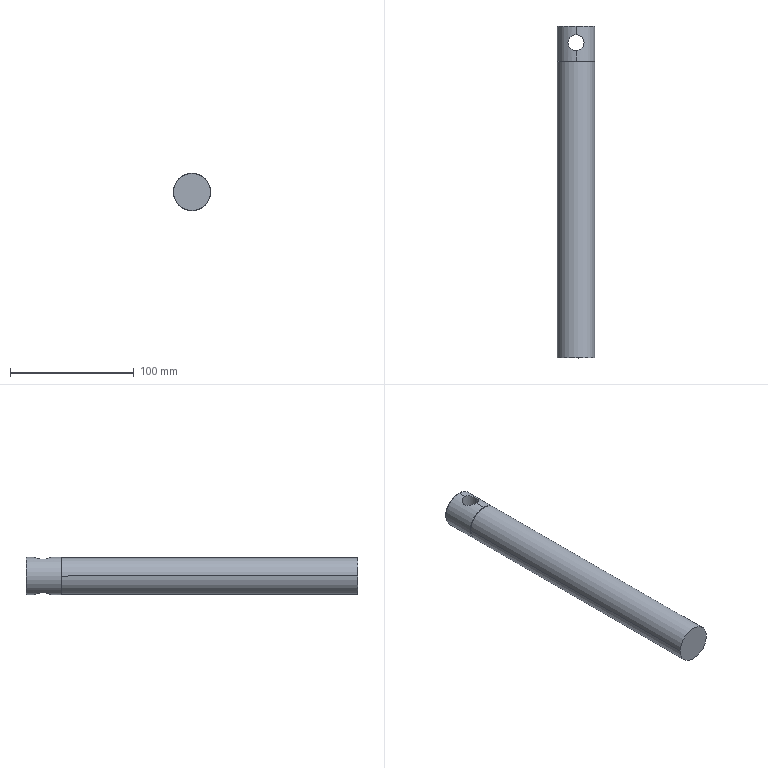Part | SolidWorks | features BaseBody 1 | 1 solid | 29 faces | box 30 x 268.629 x 30.034 mm | volume 178824 mm3 | cylinder 14 | plane 7 | cone 6 | torus 2 | commonest cylinder face diameters 26 x4 30 x4 13 x2 18 x2 24 x2
STEP:
#1=CARTESIAN_POINT('',(406.073,347.307,68.537));
#2=VERTEX_POINT('',#1);
#3=CARTESIAN_POINT('',(391.077,347.309,83.541));
#4=VERTEX_POINT('',#3);
#5=CARTESIAN_POINT('',(406.077,347.309,83.537));
#6=DIRECTION('',(-0.000000041,1.,-0.0001428));
#7=DIRECTION('',(-1.,0.,0.0002857));
#8=AXIS2_PLACEMENT_3D('',#5,#6,#7);
#9=CIRCLE('',#8,15.);
#10=EDGE_CURVE('',#2,#4,#9,.T.);
#11=ORIENTED_EDGE('',*,*,#10,.T.);
#12=CARTESIAN_POINT('',(391.577,347.809,83.541));
#13=VERTEX_POINT('',#12);
#14=CARTESIAN_POINT('',(391.577,347.309,83.541));
#15=DIRECTION('',(-0.0002857,-0.0001428,-1.));
#16=DIRECTION('',(-1.,0.,0.0002857));
#17=AXIS2_PLACEMENT_3D('',#14,#15,#16);
#18=CIRCLE('',#17,0.5);
#19=EDGE_CURVE('',#4,#13,#18,.T.);
#20=ORIENTED_EDGE('',*,*,#19,.T.);
#21=CARTESIAN_POINT('',(420.577,347.809,83.533));
#22=VERTEX_POINT('',#21);
#23=CARTESIAN_POINT('',(406.077,347.809,83.537));
#24=DIRECTION('',(-0.000000041,1.,-0.0001428));
#25=DIRECTION('',(1.,0.,-0.0002857));
#26=AXIS2_PLACEMENT_3D('',#23,#24,#25);
#27=CIRCLE('',#26,14.5);
#28=EDGE_CURVE('',#22,#13,#27,.T.);
#29=ORIENTED_EDGE('',*,*,#28,.F.);
#30=CARTESIAN_POINT('',(421.077,347.309,83.533));
#31=VERTEX_POINT('',#30);
#32=CARTESIAN_POINT('',(420.577,347.309,83.533));
#33=DIRECTION('',(0.0002857,0.0001428,1.));
#34=DIRECTION('',(1.,0.,-0.0002857));
#35=AXIS2_PLACEMENT_3D('',#32,#33,#34);
#36=CIRCLE('',#35,0.5);
#37=EDGE_CURVE('',#31,#22,#36,.T.);
#38=ORIENTED_EDGE('',*,*,#37,.F.);
#39=CARTESIAN_POINT('',(406.077,347.309,83.537));
#40=DIRECTION('',(-0.000000041,1.,-0.0001428));
#41=DIRECTION('',(-1.,0.,0.0002857));
#42=AXIS2_PLACEMENT_3D('',#39,#40,#41);
#43=CIRCLE('',#42,15.);
#44=EDGE_CURVE('',#31,#2,#43,.T.);
#45=ORIENTED_EDGE('',*,*,#44,.T.);
#46=EDGE_LOOP('',(#11,#20,#29,#38,#45));
#47=FACE_OUTER_BOUND('',#46,.T.);
#48=CARTESIAN_POINT('',(406.077,347.309,83.537));
#49=DIRECTION('',(-0.000000041,1.,-0.0001428));
#50=DIRECTION('',(1.,0.,-0.0002857));
#51=AXIS2_PLACEMENT_3D('',#48,#49,#50);
#52=TOROIDAL_SURFACE('',#51,14.5,0.5);
#53=ADVANCED_FACE('',(#47),#52,.T.);
#54=CARTESIAN_POINT('',(406.073,340.807,68.538));
#55=VERTEX_POINT('',#54);
#56=CARTESIAN_POINT('',(412.574,334.308,70.018));
#57=VERTEX_POINT('',#56);
#58=CARTESIAN_POINT('',(406.073,340.807,68.538));
#59=CARTESIAN_POINT('',(406.508,340.807,68.538));
#60=CARTESIAN_POINT('',(406.937,340.764,68.556));
#61=CARTESIAN_POINT('',(407.571,340.636,68.611));
#62=CARTESIAN_POINT('',(407.781,340.583,68.633));
#63=CARTESIAN_POINT('',(408.191,340.457,68.686));
#64=CARTESIAN_POINT('',(408.39,340.384,68.716));
#65=CARTESIAN_POINT('',(408.976,340.139,68.815));
#66=CARTESIAN_POINT('',(409.349,339.938,68.895));
#67=CARTESIAN_POINT('',(410.054,339.463,69.07));
#68=CARTESIAN_POINT('',(410.378,339.196,69.164));
#69=CARTESIAN_POINT('',(410.821,338.752,69.307));
#70=CARTESIAN_POINT('',(410.962,338.596,69.355));
#71=CARTESIAN_POINT('',(411.23,338.27,69.45));
#72=CARTESIAN_POINT('',(411.357,338.1,69.497));
#73=CARTESIAN_POINT('',(411.708,337.575,69.633));
#74=CARTESIAN_POINT('',(411.907,337.205,69.716));
#75=CARTESIAN_POINT('',(412.234,336.423,69.859));
#76=CARTESIAN_POINT('',(412.362,336.008,69.918));
#77=CARTESIAN_POINT('',(412.53,335.17,69.997));
#78=CARTESIAN_POINT('',(412.574,334.743,70.018));
#79=CARTESIAN_POINT('',(412.574,334.308,70.018));
#80=B_SPLINE_CURVE_WITH_KNOTS('',3,(#58,#59,#60,#61,#62,#63,#64,#65,#66,#67,#68,#69,#70,#71,#72,#73,#74,#75,#76,#77,#78,#79),.UNSPECIFIED.,.F.,.F.,(4,2,2,2,2,2,2,2,2,2,4),(0.01028,0.01157,0.01221,0.01285,0.01414,0.01543,0.01607,0.01671,0.018,0.01928,0.02057),.UNSPECIFIED.);
#81=EDGE_CURVE('',#55,#57,#80,.T.);
#82=ORIENTED_EDGE('',*,*,#81,.T.);
#83=CARTESIAN_POINT('',(412.581,334.311,97.055));
#84=VERTEX_POINT('',#83);
#85=CARTESIAN_POINT('',(412.573,334.307,69.287));
#86=DIRECTION('',(0.0002857,0.0001428,1.));
#87=VECTOR('',#86,1000.);
#88=LINE('',#85,#87);
#89=EDGE_CURVE('',#57,#84,#88,.T.);
#90=ORIENTED_EDGE('',*,*,#89,.T.);
#91=CARTESIAN_POINT('',(406.082,340.812,98.538));
#92=VERTEX_POINT('',#91);
#93=CARTESIAN_POINT('',(412.581,334.311,97.055));
#94=CARTESIAN_POINT('',(412.581,334.747,97.055));
#95=CARTESIAN_POINT('',(412.538,335.173,97.076));
#96=CARTESIAN_POINT('',(412.37,336.011,97.155));
#97=CARTESIAN_POINT('',(412.243,336.426,97.214));
#98=CARTESIAN_POINT('',(411.915,337.209,97.357));
#99=CARTESIAN_POINT('',(411.716,337.58,97.441));
#100=CARTESIAN_POINT('',(411.363,338.107,97.577));
#101=CARTESIAN_POINT('',(411.236,338.277,97.624));
#102=CARTESIAN_POINT('',(410.968,338.602,97.719));
#103=CARTESIAN_POINT('',(410.828,338.758,97.767));
#104=CARTESIAN_POINT('',(410.384,339.201,97.91));
#105=CARTESIAN_POINT('',(410.059,339.47,98.004));
#106=CARTESIAN_POINT('',(409.355,339.943,98.18));
#107=CARTESIAN_POINT('',(408.984,340.143,98.259));
#108=CARTESIAN_POINT('',(408.398,340.388,98.358));
#109=CARTESIAN_POINT('',(408.199,340.461,98.389));
#110=CARTESIAN_POINT('',(407.789,340.587,98.441));
#111=CARTESIAN_POINT('',(407.578,340.641,98.464));
#112=CARTESIAN_POINT('',(406.945,340.768,98.519));
#113=CARTESIAN_POINT('',(406.517,340.812,98.538));
#114=CARTESIAN_POINT('',(406.082,340.812,98.538));
#115=B_SPLINE_CURVE_WITH_KNOTS('',3,(#93,#94,#95,#96,#97,#98,#99,#100,#101,#102,#103,#104,#105,#106,#107,#108,#109,#110,#111,#112,#113,#114),.UNSPECIFIED.,.F.,.F.,(4,2,2,2,2,2,2,2,2,2,4),(-0.02056,-0.01928,-0.01799,-0.01671,-0.01606,-0.01542,-0.01414,-0.01285,-0.01221,-0.01156,-0.01028),.UNSPECIFIED.);
#116=EDGE_CURVE('',#84,#92,#115,.T.);
#117=ORIENTED_EDGE('',*,*,#116,.T.);
#118=CARTESIAN_POINT('',(399.581,334.311,97.059));
#119=VERTEX_POINT('',#118);
#120=CARTESIAN_POINT('',(406.082,340.812,98.538));
#121=CARTESIAN_POINT('',(405.647,340.812,98.538));
#122=CARTESIAN_POINT('',(405.221,340.768,98.519));
#123=CARTESIAN_POINT('',(404.592,340.642,98.466));
#124=CARTESIAN_POINT('',(404.385,340.59,98.443));
#125=CARTESIAN_POINT('',(403.974,340.464,98.391));
#126=CARTESIAN_POINT('',(403.772,340.391,98.361));
#127=CARTESIAN_POINT('',(403.183,340.145,98.261));
#128=CARTESIAN_POINT('',(402.812,339.945,98.183));
#129=CARTESIAN_POINT('',(402.11,339.474,98.008));
#130=CARTESIAN_POINT('',(401.779,339.202,97.912));
#131=CARTESIAN_POINT('',(401.184,338.606,97.721));
#132=CARTESIAN_POINT('',(400.919,338.283,97.625));
#133=CARTESIAN_POINT('',(400.451,337.586,97.445));
#134=CARTESIAN_POINT('',(400.247,337.208,97.36));
#135=CARTESIAN_POINT('',(399.921,336.427,97.218));
#136=CARTESIAN_POINT('',(399.796,336.022,97.16));
#137=CARTESIAN_POINT('',(399.668,335.392,97.1));
#138=CARTESIAN_POINT('',(399.636,335.176,97.085));
#139=CARTESIAN_POINT('',(399.592,334.745,97.064));
#140=CARTESIAN_POINT('',(399.581,334.529,97.059));
#141=CARTESIAN_POINT('',(399.581,334.311,97.059));
#142=B_SPLINE_CURVE_WITH_KNOTS('',3,(#120,#121,#122,#123,#124,#125,#126,#127,#128,#129,#130,#131,#132,#133,#134,#135,#136,#137,#138,#139,#140,#141),.UNSPECIFIED.,.F.,.F.,(4,2,2,2,2,2,2,2,2,2,4),(-0.01028,-0.008994,-0.008351,-0.007709,-0.006424,-0.005139,-0.003854,-0.00257,-0.001285,-0.0006424,0.),.UNSPECIFIED.);
#143=EDGE_CURVE('',#92,#119,#142,.T.);
#144=ORIENTED_EDGE('',*,*,#143,.T.);
#145=CARTESIAN_POINT('',(399.574,334.308,70.022));
#146=VERTEX_POINT('',#145);
#147=CARTESIAN_POINT('',(399.573,334.307,69.291));
#148=DIRECTION('',(0.0002857,0.0001428,1.));
#149=VECTOR('',#148,1000.);
#150=LINE('',#147,#149);
#151=EDGE_CURVE('',#146,#119,#150,.T.);
#152=ORIENTED_EDGE('',*,*,#151,.F.);
#153=CARTESIAN_POINT('',(399.574,334.308,70.022));
#154=CARTESIAN_POINT('',(399.574,334.743,70.022));
#155=CARTESIAN_POINT('',(399.617,335.169,70.001));
#156=CARTESIAN_POINT('',(399.785,336.007,69.922));
#157=CARTESIAN_POINT('',(399.912,336.422,69.863));
#158=CARTESIAN_POINT('',(400.24,337.205,69.72));
#159=CARTESIAN_POINT('',(400.439,337.576,69.636));
#160=CARTESIAN_POINT('',(400.792,338.103,69.5));
#161=CARTESIAN_POINT('',(400.919,338.273,69.452));
#162=CARTESIAN_POINT('',(401.186,338.598,69.357));
#163=CARTESIAN_POINT('',(401.327,338.753,69.309));
#164=CARTESIAN_POINT('',(401.771,339.197,69.166));
#165=CARTESIAN_POINT('',(402.096,339.466,69.071));
#166=CARTESIAN_POINT('',(402.8,339.939,68.896));
#167=CARTESIAN_POINT('',(403.171,340.139,68.817));
#168=CARTESIAN_POINT('',(403.757,340.384,68.717));
#169=CARTESIAN_POINT('',(403.956,340.457,68.687));
#170=CARTESIAN_POINT('',(404.366,340.583,68.634));
#171=CARTESIAN_POINT('',(404.577,340.636,68.612));
#172=CARTESIAN_POINT('',(405.21,340.764,68.557));
#173=CARTESIAN_POINT('',(405.638,340.807,68.538));
#174=CARTESIAN_POINT('',(406.073,340.807,68.538));
#175=B_SPLINE_CURVE_WITH_KNOTS('',3,(#153,#154,#155,#156,#157,#158,#159,#160,#161,#162,#163,#164,#165,#166,#167,#168,#169,#170,#171,#172,#173,#174),.UNSPECIFIED.,.F.,.F.,(4,2,2,2,2,2,2,2,2,2,4),(-0.000000012,0.001285,0.002571,0.003856,0.004499,0.005142,0.006427,0.007713,0.008355,0.008998,0.01028),.UNSPECIFIED.);
#176=EDGE_CURVE('',#146,#55,#175,.T.);
#177=ORIENTED_EDGE('',*,*,#176,.T.);
#178=EDGE_LOOP('',(#82,#90,#117,#144,#152,#177));
#179=FACE_OUTER_BOUND('',#178,.T.);
#180=CARTESIAN_POINT('',(406.073,334.307,69.289));
#181=DIRECTION('',(0.0002857,0.0001428,1.));
#182=DIRECTION('',(-1.,0.,0.0002857));
#183=AXIS2_PLACEMENT_3D('',#180,#181,#182);
#184=CYLINDRICAL_SURFACE('',#183,6.5);
#185=ADVANCED_FACE('',(#179),#184,.F.);
#186=ORIENTED_EDGE('',*,*,#10,.F.);
#187=CARTESIAN_POINT('',(406.073,336.807,68.538));
#188=DIRECTION('',(0.000000041,-1.,0.0001428));
#189=VECTOR('',#188,1000.);
#190=LINE('',#187,#189);
#191=EDGE_CURVE('',#2,#55,#190,.T.);
#192=ORIENTED_EDGE('',*,*,#191,.T.);
#193=ORIENTED_EDGE('',*,*,#176,.F.);
#194=CARTESIAN_POINT('',(406.073,327.807,68.54));
#195=VERTEX_POINT('',#194);
#196=CARTESIAN_POINT('',(406.073,327.807,68.54));
#197=CARTESIAN_POINT('',(405.638,327.807,68.54));
#198=CARTESIAN_POINT('',(405.209,327.851,68.559));
#199=CARTESIAN_POINT('',(404.575,327.979,68.613));
#200=CARTESIAN_POINT('',(404.365,328.032,68.636));
#201=CARTESIAN_POINT('',(403.956,328.158,68.689));
#202=CARTESIAN_POINT('',(403.756,328.231,68.719));
#203=CARTESIAN_POINT('',(403.17,328.476,68.819));
#204=CARTESIAN_POINT('',(402.797,328.677,68.898));
#205=CARTESIAN_POINT('',(402.092,329.152,69.074));
#206=CARTESIAN_POINT('',(401.769,329.419,69.168));
#207=CARTESIAN_POINT('',(401.326,329.863,69.311));
#208=CARTESIAN_POINT('',(401.185,330.019,69.359));
#209=CARTESIAN_POINT('',(400.917,330.345,69.454));
#210=CARTESIAN_POINT('',(400.79,330.516,69.501));
#211=CARTESIAN_POINT('',(400.439,331.04,69.637));
#212=CARTESIAN_POINT('',(400.24,331.41,69.72));
#213=CARTESIAN_POINT('',(399.913,332.192,69.863));
#214=CARTESIAN_POINT('',(399.785,332.608,69.922));
#215=CARTESIAN_POINT('',(399.617,333.446,70.001));
#216=CARTESIAN_POINT('',(399.574,333.872,70.022));
#217=CARTESIAN_POINT('',(399.574,334.308,70.022));
#218=B_SPLINE_CURVE_WITH_KNOTS('',3,(#196,#197,#198,#199,#200,#201,#202,#203,#204,#205,#206,#207,#208,#209,#210,#211,#212,#213,#214,#215,#216,#217),.UNSPECIFIED.,.F.,.F.,(4,2,2,2,2,2,2,2,2,2,4),(-0.01029,-0.009,-0.008357,-0.007714,-0.006429,-0.005143,-0.0045,-0.003857,-0.002571,-0.001286,-0.000000012),.UNSPECIFIED.);
#219=EDGE_CURVE('',#195,#146,#218,.T.);
#220=ORIENTED_EDGE('',*,*,#219,.F.);
#221=CARTESIAN_POINT('',(406.073,319.307,68.541));
#222=VERTEX_POINT('',#221);
#223=CARTESIAN_POINT('',(406.073,336.807,68.538));
#224=DIRECTION('',(0.000000041,-1.,0.0001428));
#225=VECTOR('',#224,1000.);
#226=LINE('',#223,#225);
#227=EDGE_CURVE('',#195,#222,#226,.T.);
#228=ORIENTED_EDGE('',*,*,#227,.T.);
#229=CARTESIAN_POINT('',(391.077,319.309,83.545));
#230=VERTEX_POINT('',#229);
#231=CARTESIAN_POINT('',(406.077,319.309,83.541));
#232=DIRECTION('',(0.000000041,-1.,0.0001428));
#233=DIRECTION('',(-0.0002857,-0.0001428,-1.));
#234=AXIS2_PLACEMENT_3D('',#231,#232,#233);
#235=CIRCLE('',#234,15.);
#236=EDGE_CURVE('',#230,#222,#235,.T.);
#237=ORIENTED_EDGE('',*,*,#236,.F.);
#238=CARTESIAN_POINT('',(406.082,319.312,98.541));
#239=VERTEX_POINT('',#238);
#240=CARTESIAN_POINT('',(406.077,319.309,83.541));
#241=DIRECTION('',(0.000000041,-1.,0.0001428));
#242=DIRECTION('',(-0.0002857,-0.0001428,-1.));
#243=AXIS2_PLACEMENT_3D('',#240,#241,#242);
#244=CIRCLE('',#243,15.);
#245=EDGE_CURVE('',#239,#230,#244,.T.);
#246=ORIENTED_EDGE('',*,*,#245,.F.);
#247=CARTESIAN_POINT('',(406.082,327.812,98.54));
#248=VERTEX_POINT('',#247);
#249=CARTESIAN_POINT('',(406.082,336.812,98.538));
#250=DIRECTION('',(0.000000041,-1.,0.0001428));
#251=VECTOR('',#250,1000.);
#252=LINE('',#249,#251);
#253=EDGE_CURVE('',#248,#239,#252,.T.);
#254=ORIENTED_EDGE('',*,*,#253,.F.);
#255=CARTESIAN_POINT('',(399.581,334.311,97.059));
#256=CARTESIAN_POINT('',(399.581,333.876,97.059));
#257=CARTESIAN_POINT('',(399.625,333.45,97.08));
#258=CARTESIAN_POINT('',(399.793,332.612,97.159));
#259=CARTESIAN_POINT('',(399.92,332.197,97.218));
#260=CARTESIAN_POINT('',(400.248,331.414,97.361));
#261=CARTESIAN_POINT('',(400.447,331.043,97.445));
#262=CARTESIAN_POINT('',(400.8,330.516,97.581));
#263=CARTESIAN_POINT('',(400.927,330.346,97.628));
#264=CARTESIAN_POINT('',(401.195,330.021,97.723));
#265=CARTESIAN_POINT('',(401.335,329.866,97.771));
#266=CARTESIAN_POINT('',(401.779,329.422,97.914));
#267=CARTESIAN_POINT('',(402.104,329.153,98.008));
#268=CARTESIAN_POINT('',(402.809,328.68,98.183));
#269=CARTESIAN_POINT('',(403.18,328.48,98.262));
#270=CARTESIAN_POINT('',(403.765,328.235,98.362));
#271=CARTESIAN_POINT('',(403.965,328.162,98.391));
#272=CARTESIAN_POINT('',(404.375,328.036,98.444));
#273=CARTESIAN_POINT('',(404.585,327.983,98.467));
#274=CARTESIAN_POINT('',(405.218,327.855,98.521));
#275=CARTESIAN_POINT('',(405.647,327.812,98.54));
#276=CARTESIAN_POINT('',(406.082,327.812,98.54));
#277=B_SPLINE_CURVE_WITH_KNOTS('',3,(#255,#256,#257,#258,#259,#260,#261,#262,#263,#264,#265,#266,#267,#268,#269,#270,#271,#272,#273,#274,#275,#276),.UNSPECIFIED.,.F.,.F.,(4,2,2,2,2,2,2,2,2,2,4),(0.,0.001285,0.002571,0.003856,0.004499,0.005142,0.006427,0.007713,0.008355,0.008998,0.01028),.UNSPECIFIED.);
#278=EDGE_CURVE('',#119,#248,#277,.T.);
#279=ORIENTED_EDGE('',*,*,#278,.F.);
#280=ORIENTED_EDGE('',*,*,#143,.F.);
#281=CARTESIAN_POINT('',(406.082,347.312,98.537));
#282=VERTEX_POINT('',#281);
#283=CARTESIAN_POINT('',(406.082,336.812,98.538));
#284=DIRECTION('',(0.000000041,-1.,0.0001428));
#285=VECTOR('',#284,1000.);
#286=LINE('',#283,#285);
#287=EDGE_CURVE('',#282,#92,#286,.T.);
#288=ORIENTED_EDGE('',*,*,#287,.F.);
#289=CARTESIAN_POINT('',(406.077,347.309,83.537));
#290=DIRECTION('',(-0.000000041,1.,-0.0001428));
#291=DIRECTION('',(-1.,0.,0.0002857));
#292=AXIS2_PLACEMENT_3D('',#289,#290,#291);
#293=CIRCLE('',#292,15.);
#294=EDGE_CURVE('',#4,#282,#293,.T.);
#295=ORIENTED_EDGE('',*,*,#294,.F.);
#296=EDGE_LOOP('',(#186,#192,#193,#220,#228,#237,#246,#254,#279,#280,#288,#295));
#297=FACE_OUTER_BOUND('',#296,.T.);
#298=CARTESIAN_POINT('',(406.077,336.809,83.538));
#299=DIRECTION('',(0.000000041,-1.,0.0001428));
#300=DIRECTION('',(0.0002857,0.0001428,1.));
#301=AXIS2_PLACEMENT_3D('',#298,#299,#300);
#302=CYLINDRICAL_SURFACE('',#301,15.);
#303=ADVANCED_FACE('',(#297),#302,.T.);
#304=CARTESIAN_POINT('',(391.577,318.809,83.545));
#305=VERTEX_POINT('',#304);
#306=CARTESIAN_POINT('',(420.577,318.809,83.537));
#307=VERTEX_POINT('',#306);
#308=CARTESIAN_POINT('',(406.077,318.809,83.541));
#309=DIRECTION('',(0.000000041,-1.,0.0001428));
#310=DIRECTION('',(1.,0.,-0.0002857));
#311=AXIS2_PLACEMENT_3D('',#308,#309,#310);
#312=CIRCLE('',#311,14.5);
#313=EDGE_CURVE('',#305,#307,#312,.T.);
#314=ORIENTED_EDGE('',*,*,#313,.F.);
#315=CARTESIAN_POINT('',(391.327,319.059,83.545));
#316=DIRECTION('',(-0.7071,0.7071,0.000101));
#317=VECTOR('',#316,1000.);
#318=LINE('',#315,#317);
#319=EDGE_CURVE('',#305,#230,#318,.T.);
#320=ORIENTED_EDGE('',*,*,#319,.T.);
#321=ORIENTED_EDGE('',*,*,#236,.T.);
#322=CARTESIAN_POINT('',(421.077,319.309,83.537));
#323=VERTEX_POINT('',#322);
#324=CARTESIAN_POINT('',(406.077,319.309,83.541));
#325=DIRECTION('',(0.000000041,-1.,0.0001428));
#326=DIRECTION('',(-0.0002857,-0.0001428,-1.));
#327=AXIS2_PLACEMENT_3D('',#324,#325,#326);
#328=CIRCLE('',#327,15.);
#329=EDGE_CURVE('',#222,#323,#328,.T.);
#330=ORIENTED_EDGE('',*,*,#329,.T.);
#331=CARTESIAN_POINT('',(420.827,319.059,83.537));
#332=DIRECTION('',(0.7071,0.7071,-0.000303));
#333=VECTOR('',#332,1000.);
#334=LINE('',#331,#333);
#335=EDGE_CURVE('',#307,#323,#334,.T.);
#336=ORIENTED_EDGE('',*,*,#335,.F.);
#337=EDGE_LOOP('',(#314,#320,#321,#330,#336));
#338=FACE_OUTER_BOUND('',#337,.T.);
#339=CARTESIAN_POINT('',(406.077,319.059,83.541));
#340=DIRECTION('',(-0.000000041,1.,-0.0001428));
#341=DIRECTION('',(1.,0.,-0.0002857));
#342=AXIS2_PLACEMENT_3D('',#339,#340,#341);
#343=CONICAL_SURFACE('',#342,14.75,0.7854);
#344=ADVANCED_FACE('',(#338),#343,.T.);
#345=CARTESIAN_POINT('',(421.077,79.185,83.564));
#346=VERTEX_POINT('',#345);
#347=CARTESIAN_POINT('',(391.077,79.185,83.572));
#348=VERTEX_POINT('',#347);
#349=CARTESIAN_POINT('',(406.077,79.185,83.568));
#350=DIRECTION('',(0.000000041,-1.,0.0001428));
#351=DIRECTION('',(-1.,0.,0.0002857));
#352=AXIS2_PLACEMENT_3D('',#349,#350,#351);
#353=CIRCLE('',#352,15.);
#354=EDGE_CURVE('',#346,#348,#353,.T.);
#355=ORIENTED_EDGE('',*,*,#354,.F.);
#356=CARTESIAN_POINT('',(421.077,318.809,83.529));
#357=VERTEX_POINT('',#356);
#358=CARTESIAN_POINT('',(421.077,95.935,83.561));
#359=DIRECTION('',(-0.000000041,1.,-0.0001428));
#360=VECTOR('',#359,1000.);
#361=LINE('',#358,#360);
#362=EDGE_CURVE('',#346,#357,#361,.T.);
#363=ORIENTED_EDGE('',*,*,#362,.T.);
#364=CARTESIAN_POINT('',(391.077,318.809,83.538));
#365=VERTEX_POINT('',#364);
#366=CARTESIAN_POINT('',(406.077,318.809,83.534));
#367=DIRECTION('',(-0.000000041,1.,-0.0001428));
#368=DIRECTION('',(1.,0.,-0.0002857));
#369=AXIS2_PLACEMENT_3D('',#366,#367,#368);
#370=CIRCLE('',#369,15.);
#371=EDGE_CURVE('',#365,#357,#370,.T.);
#372=ORIENTED_EDGE('',*,*,#371,.F.);
#373=CARTESIAN_POINT('',(391.077,95.935,83.57));
#374=DIRECTION('',(-0.000000041,1.,-0.0001428));
#375=VECTOR('',#374,1000.);
#376=LINE('',#373,#375);
#377=EDGE_CURVE('',#348,#365,#376,.T.);
#378=ORIENTED_EDGE('',*,*,#377,.F.);
#379=EDGE_LOOP('',(#355,#363,#372,#378));
#380=FACE_OUTER_BOUND('',#379,.T.);
#381=CARTESIAN_POINT('',(406.077,95.935,83.566));
#382=DIRECTION('',(-0.000000041,1.,-0.0001428));
#383=DIRECTION('',(-1.,0.,0.0002857));
#384=AXIS2_PLACEMENT_3D('',#381,#382,#383);
#385=CYLINDRICAL_SURFACE('',#384,15.);
#386=ADVANCED_FACE('',(#380),#385,.T.);
#387=ORIENTED_EDGE('',*,*,#362,.F.);
#388=CARTESIAN_POINT('',(406.077,79.185,83.568));
#389=DIRECTION('',(0.000000041,-1.,0.0001428));
#390=DIRECTION('',(-1.,0.,0.0002857));
#391=AXIS2_PLACEMENT_3D('',#388,#389,#390);
#392=CIRCLE('',#391,15.);
#393=EDGE_CURVE('',#348,#346,#392,.T.);
#394=ORIENTED_EDGE('',*,*,#393,.F.);
#395=ORIENTED_EDGE('',*,*,#377,.T.);
#396=CARTESIAN_POINT('',(406.077,318.809,83.534));
#397=DIRECTION('',(-0.000000041,1.,-0.0001428));
#398=DIRECTION('',(1.,0.,-0.0002857));
#399=AXIS2_PLACEMENT_3D('',#396,#397,#398);
#400=CIRCLE('',#399,15.);
#401=EDGE_CURVE('',#357,#365,#400,.T.);
#402=ORIENTED_EDGE('',*,*,#401,.F.);
#403=EDGE_LOOP('',(#387,#394,#395,#402));
#404=FACE_OUTER_BOUND('',#403,.T.);
#405=CARTESIAN_POINT('',(406.077,95.935,83.566));
#406=DIRECTION('',(-0.000000041,1.,-0.0001428));
#407=DIRECTION('',(-1.,0.,0.0002857));
#408=AXIS2_PLACEMENT_3D('',#405,#406,#407);
#409=CYLINDRICAL_SURFACE('',#408,15.);
#410=ADVANCED_FACE('',(#404),#409,.T.);
#411=ORIENTED_EDGE('',*,*,#371,.T.);
#412=ORIENTED_EDGE('',*,*,#401,.T.);
#413=EDGE_LOOP('',(#411,#412));
#414=FACE_OUTER_BOUND('',#413,.T.);
#415=CARTESIAN_POINT('',(406.077,318.809,83.541));
#416=DIRECTION('',(0.000000041,-1.,0.0001428));
#417=DIRECTION('',(1.,0.,-0.0002857));
#418=AXIS2_PLACEMENT_3D('',#415,#416,#417);
#419=CIRCLE('',#418,14.5);
#420=EDGE_CURVE('',#307,#305,#419,.T.);
#421=ORIENTED_EDGE('',*,*,#420,.T.);
#422=ORIENTED_EDGE('',*,*,#313,.T.);
#423=EDGE_LOOP('',(#421,#422));
#424=FACE_BOUND('',#423,.T.);
#425=CARTESIAN_POINT('',(406.077,318.809,83.541));
#426=DIRECTION('',(-0.000000041,1.,-0.0001428));
#427=DIRECTION('',(-1.,0.,0.0002857));
#428=AXIS2_PLACEMENT_3D('',#425,#426,#427);
#429=PLANE('',#428);
#430=ADVANCED_FACE('',(#414,#424),#429,.T.);
#431=ORIENTED_EDGE('',*,*,#319,.F.);
#432=ORIENTED_EDGE('',*,*,#420,.F.);
#433=ORIENTED_EDGE('',*,*,#335,.T.);
#434=CARTESIAN_POINT('',(406.077,319.309,83.541));
#435=DIRECTION('',(0.000000041,-1.,0.0001428));
#436=DIRECTION('',(-0.0002857,-0.0001428,-1.));
#437=AXIS2_PLACEMENT_3D('',#434,#435,#436);
#438=CIRCLE('',#437,15.);
#439=EDGE_CURVE('',#323,#239,#438,.T.);
#440=ORIENTED_EDGE('',*,*,#439,.T.);
#441=ORIENTED_EDGE('',*,*,#245,.T.);
#442=EDGE_LOOP('',(#431,#432,#433,#440,#441));
#443=FACE_OUTER_BOUND('',#442,.T.);
#444=CARTESIAN_POINT('',(406.077,319.059,83.541));
#445=DIRECTION('',(-0.000000041,1.,-0.0001428));
#446=DIRECTION('',(1.,0.,-0.0002857));
#447=AXIS2_PLACEMENT_3D('',#444,#445,#446);
#448=CONICAL_SURFACE('',#447,14.75,0.7854);
#449=ADVANCED_FACE('',(#443),#448,.T.);
#450=ORIENTED_EDGE('',*,*,#191,.F.);
#451=ORIENTED_EDGE('',*,*,#44,.F.);
#452=CARTESIAN_POINT('',(406.077,347.309,83.537));
#453=DIRECTION('',(-0.000000041,1.,-0.0001428));
#454=DIRECTION('',(-1.,0.,0.0002857));
#455=AXIS2_PLACEMENT_3D('',#452,#453,#454);
#456=CIRCLE('',#455,15.);
#457=EDGE_CURVE('',#282,#31,#456,.T.);
#458=ORIENTED_EDGE('',*,*,#457,.F.);
#459=ORIENTED_EDGE('',*,*,#287,.T.);
#460=ORIENTED_EDGE('',*,*,#116,.F.);
#461=CARTESIAN_POINT('',(406.082,327.812,98.54));
#462=CARTESIAN_POINT('',(406.517,327.812,98.539));
#463=CARTESIAN_POINT('',(406.943,327.855,98.52));
#464=CARTESIAN_POINT('',(407.571,327.981,98.466));
#465=CARTESIAN_POINT('',(407.778,328.033,98.444));
#466=CARTESIAN_POINT('',(408.189,328.159,98.392));
#467=CARTESIAN_POINT('',(408.392,328.232,98.361));
#468=CARTESIAN_POINT('',(408.98,328.478,98.261));
#469=CARTESIAN_POINT('',(409.351,328.678,98.182));
#470=CARTESIAN_POINT('',(410.054,329.149,98.007));
#471=CARTESIAN_POINT('',(410.384,329.421,97.911));
#472=CARTESIAN_POINT('',(410.979,330.017,97.719));
#473=CARTESIAN_POINT('',(411.244,330.34,97.624));
#474=CARTESIAN_POINT('',(411.712,331.037,97.443));
#475=CARTESIAN_POINT('',(411.916,331.415,97.357));
#476=CARTESIAN_POINT('',(412.242,332.196,97.215));
#477=CARTESIAN_POINT('',(412.367,332.6,97.157));
#478=CARTESIAN_POINT('',(412.495,333.231,97.097));
#479=CARTESIAN_POINT('',(412.527,333.446,97.081));
#480=CARTESIAN_POINT('',(412.57,333.877,97.061));
#481=CARTESIAN_POINT('',(412.581,334.094,97.055));
#482=CARTESIAN_POINT('',(412.581,334.311,97.055));
#483=B_SPLINE_CURVE_WITH_KNOTS('',3,(#461,#462,#463,#464,#465,#466,#467,#468,#469,#470,#471,#472,#473,#474,#475,#476,#477,#478,#479,#480,#481,#482),.UNSPECIFIED.,.F.,.F.,(4,2,2,2,2,2,2,2,2,2,4),(0.01028,0.01157,0.01221,0.01285,0.01414,0.01542,0.01671,0.01799,0.01927,0.01992,0.02056),.UNSPECIFIED.);
#484=EDGE_CURVE('',#248,#84,#483,.T.);
#485=ORIENTED_EDGE('',*,*,#484,.F.);
#486=ORIENTED_EDGE('',*,*,#253,.T.);
#487=ORIENTED_EDGE('',*,*,#439,.F.);
#488=ORIENTED_EDGE('',*,*,#329,.F.);
#489=ORIENTED_EDGE('',*,*,#227,.F.);
#490=CARTESIAN_POINT('',(412.574,334.308,70.018));
#491=CARTESIAN_POINT('',(412.574,333.872,70.018));
#492=CARTESIAN_POINT('',(412.53,333.446,69.997));
#493=CARTESIAN_POINT('',(412.362,332.608,69.919));
#494=CARTESIAN_POINT('',(412.235,332.193,69.86));
#495=CARTESIAN_POINT('',(411.907,331.41,69.717));
#496=CARTESIAN_POINT('',(411.708,331.039,69.634));
#497=CARTESIAN_POINT('',(411.355,330.512,69.498));
#498=CARTESIAN_POINT('',(411.228,330.342,69.45));
#499=CARTESIAN_POINT('',(410.96,330.017,69.356));
#500=CARTESIAN_POINT('',(410.82,329.861,69.308));
#501=CARTESIAN_POINT('',(410.376,329.418,69.165));
#502=CARTESIAN_POINT('',(410.051,329.149,69.071));
#503=CARTESIAN_POINT('',(409.346,328.675,68.895));
#504=CARTESIAN_POINT('',(408.975,328.476,68.817));
#505=CARTESIAN_POINT('',(408.39,328.231,68.718));
#506=CARTESIAN_POINT('',(408.19,328.158,68.688));
#507=CARTESIAN_POINT('',(407.78,328.032,68.635));
#508=CARTESIAN_POINT('',(407.57,327.978,68.612));
#509=CARTESIAN_POINT('',(406.937,327.851,68.558));
#510=CARTESIAN_POINT('',(406.508,327.807,68.539));
#511=CARTESIAN_POINT('',(406.073,327.807,68.54));
#512=B_SPLINE_CURVE_WITH_KNOTS('',3,(#490,#491,#492,#493,#494,#495,#496,#497,#498,#499,#500,#501,#502,#503,#504,#505,#506,#507,#508,#509,#510,#511),.UNSPECIFIED.,.F.,.F.,(4,2,2,2,2,2,2,2,2,2,4),(0.02057,0.02185,0.02314,0.02442,0.02507,0.02571,0.027,0.02828,0.02892,0.02957,0.03085),.UNSPECIFIED.);
#513=EDGE_CURVE('',#57,#195,#512,.T.);
#514=ORIENTED_EDGE('',*,*,#513,.F.);
#515=ORIENTED_EDGE('',*,*,#81,.F.);
#516=EDGE_LOOP('',(#450,#451,#458,#459,#460,#485,#486,#487,#488,#489,#514,#515));
#517=FACE_OUTER_BOUND('',#516,.T.);
#518=CARTESIAN_POINT('',(406.077,336.809,83.538));
#519=DIRECTION('',(0.000000041,-1.,0.0001428));
#520=DIRECTION('',(0.0002857,0.0001428,1.));
#521=AXIS2_PLACEMENT_3D('',#518,#519,#520);
#522=CYLINDRICAL_SURFACE('',#521,15.);
#523=ADVANCED_FACE('',(#517),#522,.T.);
#524=ORIENTED_EDGE('',*,*,#89,.F.);
#525=ORIENTED_EDGE('',*,*,#513,.T.);
#526=ORIENTED_EDGE('',*,*,#219,.T.);
#527=ORIENTED_EDGE('',*,*,#151,.T.);
#528=ORIENTED_EDGE('',*,*,#278,.T.);
#529=ORIENTED_EDGE('',*,*,#484,.T.);
#530=EDGE_LOOP('',(#524,#525,#526,#527,#528,#529));
#531=FACE_OUTER_BOUND('',#530,.T.);
#532=CARTESIAN_POINT('',(406.073,334.307,69.289));
#533=DIRECTION('',(0.0002857,0.0001428,1.));
#534=DIRECTION('',(-1.,0.,0.0002857));
#535=AXIS2_PLACEMENT_3D('',#532,#533,#534);
#536=CYLINDRICAL_SURFACE('',#535,6.5);
#537=ADVANCED_FACE('',(#531),#536,.F.);
#538=ORIENTED_EDGE('',*,*,#19,.F.);
#539=ORIENTED_EDGE('',*,*,#294,.T.);
#540=ORIENTED_EDGE('',*,*,#457,.T.);
#541=ORIENTED_EDGE('',*,*,#37,.T.);
#542=CARTESIAN_POINT('',(406.077,347.809,83.537));
#543=DIRECTION('',(-0.000000041,1.,-0.0001428));
#544=DIRECTION('',(1.,0.,-0.0002857));
#545=AXIS2_PLACEMENT_3D('',#542,#543,#544);
#546=CIRCLE('',#545,14.5);
#547=EDGE_CURVE('',#13,#22,#546,.T.);
#548=ORIENTED_EDGE('',*,*,#547,.F.);
#549=EDGE_LOOP('',(#538,#539,#540,#541,#548));
#550=FACE_OUTER_BOUND('',#549,.T.);
#551=CARTESIAN_POINT('',(406.077,347.309,83.537));
#552=DIRECTION('',(-0.000000041,1.,-0.0001428));
#553=DIRECTION('',(1.,0.,-0.0002857));
#554=AXIS2_PLACEMENT_3D('',#551,#552,#553);
#555=TOROIDAL_SURFACE('',#554,14.5,0.5);
#556=ADVANCED_FACE('',(#550),#555,.T.);
#557=ORIENTED_EDGE('',*,*,#28,.T.);
#558=ORIENTED_EDGE('',*,*,#547,.T.);
#559=EDGE_LOOP('',(#557,#558));
#560=FACE_OUTER_BOUND('',#559,.T.);
#561=CARTESIAN_POINT('',(406.077,347.809,83.537));
#562=DIRECTION('',(-0.000000041,1.,-0.0001428));
#563=DIRECTION('',(-1.,0.,0.0002857));
#564=AXIS2_PLACEMENT_3D('',#561,#562,#563);
#565=PLANE('',#564);
#566=ADVANCED_FACE('',(#560),#565,.T.);
#567=ORIENTED_EDGE('',*,*,#393,.T.);
#568=ORIENTED_EDGE('',*,*,#354,.T.);
#569=EDGE_LOOP('',(#567,#568));
#570=FACE_OUTER_BOUND('',#569,.T.);
#571=CARTESIAN_POINT('',(406.077,79.185,83.568));
#572=DIRECTION('',(0.000000041,-1.,0.0001428));
#573=DIRECTION('',(-1.,-0.000000041,0.));
#574=AXIS2_PLACEMENT_3D('',#571,#572,#573);
#575=PLANE('',#574);
#576=ADVANCED_FACE('',(#570),#575,.T.);
#577=CLOSED_SHELL('',(#53,#185,#303,#344,#386,#410,#430,#449,#523,#537,#556,#566,#576));
#578=CARTESIAN_POINT('',(393.077,291.309,83.549));
#579=VERTEX_POINT('',#578);
#580=CARTESIAN_POINT('',(419.077,291.309,83.541));
#581=VERTEX_POINT('',#580);
#582=CARTESIAN_POINT('',(406.077,291.309,83.545));
#583=DIRECTION('',(-0.000000041,1.,-0.0001428));
#584=DIRECTION('',(-1.,0.,0.0002857));
#585=AXIS2_PLACEMENT_3D('',#582,#583,#584);
#586=CIRCLE('',#585,13.);
#587=EDGE_CURVE('',#579,#581,#586,.T.);
#588=ORIENTED_EDGE('',*,*,#587,.F.);
#589=CARTESIAN_POINT('',(393.077,299.309,83.547));
#590=VERTEX_POINT('',#589);
#591=CARTESIAN_POINT('',(393.077,-123.291,83.608));
#592=DIRECTION('',(-0.000000041,1.,-0.0001428));
#593=VECTOR('',#592,1000.);
#594=LINE('',#591,#593);
#595=EDGE_CURVE('',#579,#590,#594,.T.);
#596=ORIENTED_EDGE('',*,*,#595,.T.);
#597=CARTESIAN_POINT('',(419.077,299.309,83.54));
#598=VERTEX_POINT('',#597);
#599=CARTESIAN_POINT('',(406.077,299.309,83.544));
#600=DIRECTION('',(0.000000041,-1.,0.0001428));
#601=DIRECTION('',(-1.,0.,0.0002857));
#602=AXIS2_PLACEMENT_3D('',#599,#600,#601);
#603=CIRCLE('',#602,13.);
#604=EDGE_CURVE('',#598,#590,#603,.T.);
#605=ORIENTED_EDGE('',*,*,#604,.F.);
#606=CARTESIAN_POINT('',(419.077,-123.291,83.6));
#607=DIRECTION('',(-0.000000041,1.,-0.0001428));
#608=VECTOR('',#607,1000.);
#609=LINE('',#606,#608);
#610=EDGE_CURVE('',#581,#598,#609,.T.);
#611=ORIENTED_EDGE('',*,*,#610,.F.);
#612=EDGE_LOOP('',(#588,#596,#605,#611));
#613=FACE_OUTER_BOUND('',#612,.T.);
#614=CARTESIAN_POINT('',(406.077,-123.291,83.604));
#615=DIRECTION('',(-0.000000041,1.,-0.0001428));
#616=DIRECTION('',(1.,0.,-0.0002857));
#617=AXIS2_PLACEMENT_3D('',#614,#615,#616);
#618=CYLINDRICAL_SURFACE('',#617,13.);
#619=ADVANCED_FACE('',(#613),#618,.F.);
#620=CARTESIAN_POINT('',(393.577,298.809,83.547));
#621=VERTEX_POINT('',#620);
#622=CARTESIAN_POINT('',(418.577,298.809,83.54));
#623=VERTEX_POINT('',#622);
#624=CARTESIAN_POINT('',(406.077,298.809,83.544));
#625=DIRECTION('',(0.000000041,-1.,0.0001428));
#626=DIRECTION('',(-1.,0.,0.0002857));
#627=AXIS2_PLACEMENT_3D('',#624,#625,#626);
#628=CIRCLE('',#627,12.5);
#629=EDGE_CURVE('',#621,#623,#628,.T.);
#630=ORIENTED_EDGE('',*,*,#629,.F.);
#631=CARTESIAN_POINT('',(393.327,299.059,83.547));
#632=DIRECTION('',(-0.7071,0.7071,0.000101));
#633=VECTOR('',#632,1000.);
#634=LINE('',#631,#633);
#635=EDGE_CURVE('',#621,#590,#634,.T.);
#636=ORIENTED_EDGE('',*,*,#635,.T.);
#637=CARTESIAN_POINT('',(406.077,299.309,83.544));
#638=DIRECTION('',(0.000000041,-1.,0.0001428));
#639=DIRECTION('',(-1.,0.,0.0002857));
#640=AXIS2_PLACEMENT_3D('',#637,#638,#639);
#641=CIRCLE('',#640,13.);
#642=EDGE_CURVE('',#590,#598,#641,.T.);
#643=ORIENTED_EDGE('',*,*,#642,.T.);
#644=CARTESIAN_POINT('',(418.827,299.059,83.54));
#645=DIRECTION('',(0.7071,0.7071,-0.000303));
#646=VECTOR('',#645,1000.);
#647=LINE('',#644,#646);
#648=EDGE_CURVE('',#623,#598,#647,.T.);
#649=ORIENTED_EDGE('',*,*,#648,.F.);
#650=EDGE_LOOP('',(#630,#636,#643,#649));
#651=FACE_OUTER_BOUND('',#650,.T.);
#652=CARTESIAN_POINT('',(406.077,299.059,83.544));
#653=DIRECTION('',(-0.000000041,1.,-0.0001428));
#654=DIRECTION('',(1.,0.,-0.0002857));
#655=AXIS2_PLACEMENT_3D('',#652,#653,#654);
#656=CONICAL_SURFACE('',#655,12.75,0.7854);
#657=ADVANCED_FACE('',(#651),#656,.T.);
#658=CARTESIAN_POINT('',(406.075,308.808,74.542));
#659=VERTEX_POINT('',#658);
#660=CARTESIAN_POINT('',(406.08,308.811,92.542));
#661=VERTEX_POINT('',#660);
#662=CARTESIAN_POINT('',(406.077,308.809,83.542));
#663=DIRECTION('',(0.000000041,-1.,0.0001428));
#664=DIRECTION('',(0.0002857,0.0001428,1.));
#665=AXIS2_PLACEMENT_3D('',#662,#663,#664);
#666=CIRCLE('',#665,9.);
#667=EDGE_CURVE('',#659,#661,#666,.T.);
#668=ORIENTED_EDGE('',*,*,#667,.F.);
#669=CARTESIAN_POINT('',(406.075,298.808,74.544));
#670=VERTEX_POINT('',#669);
#671=CARTESIAN_POINT('',(406.075,298.808,74.544));
#672=DIRECTION('',(0.000000041,-1.,0.0001428));
#673=VECTOR('',#672,1000.);
#674=LINE('',#671,#673);
#675=EDGE_CURVE('',#659,#670,#674,.T.);
#676=ORIENTED_EDGE('',*,*,#675,.T.);
#677=CARTESIAN_POINT('',(406.08,298.811,92.544));
#678=VERTEX_POINT('',#677);
#679=CARTESIAN_POINT('',(406.077,298.809,83.544));
#680=DIRECTION('',(-0.000000041,1.,-0.0001428));
#681=DIRECTION('',(-0.0002857,-0.0001428,-1.));
#682=AXIS2_PLACEMENT_3D('',#679,#680,#681);
#683=CIRCLE('',#682,9.);
#684=EDGE_CURVE('',#678,#670,#683,.T.);
#685=ORIENTED_EDGE('',*,*,#684,.F.);
#686=CARTESIAN_POINT('',(406.08,298.811,92.544));
#687=DIRECTION('',(0.000000041,-1.,0.0001428));
#688=VECTOR('',#687,1000.);
#689=LINE('',#686,#688);
#690=EDGE_CURVE('',#661,#678,#689,.T.);
#691=ORIENTED_EDGE('',*,*,#690,.F.);
#692=EDGE_LOOP('',(#668,#676,#685,#691));
#693=FACE_OUTER_BOUND('',#692,.T.);
#694=CARTESIAN_POINT('',(406.077,298.809,83.544));
#695=DIRECTION('',(0.000000041,-1.,0.0001428));
#696=DIRECTION('',(0.0002857,0.0001428,1.));
#697=AXIS2_PLACEMENT_3D('',#694,#695,#696);
#698=CYLINDRICAL_SURFACE('',#697,9.);
#699=ADVANCED_FACE('',(#693),#698,.F.);
#700=CARTESIAN_POINT('',(406.077,314.217,83.542));
#701=VERTEX_POINT('',#700);
#702=CARTESIAN_POINT('',(406.076,311.429,78.902));
#703=DIRECTION('',(-0.0002448,-0.5152,-0.8571));
#704=VECTOR('',#703,1000.);
#705=LINE('',#702,#704);
#706=EDGE_CURVE('',#701,#659,#705,.T.);
#707=ORIENTED_EDGE('',*,*,#706,.F.);
#708=CARTESIAN_POINT('',(406.079,311.43,88.182));
#709=DIRECTION('',(0.0002449,-0.5149,0.8572));
#710=VECTOR('',#709,1000.);
#711=LINE('',#708,#710);
#712=EDGE_CURVE('',#701,#661,#711,.T.);
#713=ORIENTED_EDGE('',*,*,#712,.T.);
#714=CARTESIAN_POINT('',(406.077,308.809,83.542));
#715=DIRECTION('',(0.000000041,-1.,0.0001428));
#716=DIRECTION('',(0.0002857,0.0001428,1.));
#717=AXIS2_PLACEMENT_3D('',#714,#715,#716);
#718=CIRCLE('',#717,9.);
#719=EDGE_CURVE('',#661,#659,#718,.T.);
#720=ORIENTED_EDGE('',*,*,#719,.T.);
#721=EDGE_LOOP('',(#707,#713,#720));
#722=FACE_OUTER_BOUND('',#721,.T.);
#723=CARTESIAN_POINT('',(406.077,311.429,83.542));
#724=DIRECTION('',(0.000000041,-1.,0.0001428));
#725=DIRECTION('',(-0.0002857,-0.0001428,-1.));
#726=AXIS2_PLACEMENT_3D('',#723,#724,#725);
#727=CONICAL_SURFACE('',#726,4.64,1.03);
#728=ADVANCED_FACE('',(#722),#727,.F.);
#729=ORIENTED_EDGE('',*,*,#712,.F.);
#730=ORIENTED_EDGE('',*,*,#706,.T.);
#731=ORIENTED_EDGE('',*,*,#667,.T.);
#732=EDGE_LOOP('',(#729,#730,#731));
#733=FACE_OUTER_BOUND('',#732,.T.);
#734=CARTESIAN_POINT('',(406.077,311.429,83.542));
#735=DIRECTION('',(0.000000041,-1.,0.0001428));
#736=DIRECTION('',(-0.0002857,-0.0001428,-1.));
#737=AXIS2_PLACEMENT_3D('',#734,#735,#736);
#738=CONICAL_SURFACE('',#737,4.64,1.03);
#739=ADVANCED_FACE('',(#733),#738,.F.);
#740=ORIENTED_EDGE('',*,*,#675,.F.);
#741=ORIENTED_EDGE('',*,*,#719,.F.);
#742=ORIENTED_EDGE('',*,*,#690,.T.);
#743=CARTESIAN_POINT('',(406.077,298.809,83.544));
#744=DIRECTION('',(-0.000000041,1.,-0.0001428));
#745=DIRECTION('',(-0.0002857,-0.0001428,-1.));
#746=AXIS2_PLACEMENT_3D('',#743,#744,#745);
#747=CIRCLE('',#746,9.);
#748=EDGE_CURVE('',#670,#678,#747,.T.);
#749=ORIENTED_EDGE('',*,*,#748,.F.);
#750=EDGE_LOOP('',(#740,#741,#742,#749));
#751=FACE_OUTER_BOUND('',#750,.T.);
#752=CARTESIAN_POINT('',(406.077,298.809,83.544));
#753=DIRECTION('',(0.000000041,-1.,0.0001428));
#754=DIRECTION('',(0.0002857,0.0001428,1.));
#755=AXIS2_PLACEMENT_3D('',#752,#753,#754);
#756=CYLINDRICAL_SURFACE('',#755,9.);
#757=ADVANCED_FACE('',(#751),#756,.F.);
#758=CARTESIAN_POINT('',(406.077,298.809,83.544));
#759=DIRECTION('',(0.000000041,-1.,0.0001428));
#760=DIRECTION('',(-1.,0.,0.0002857));
#761=AXIS2_PLACEMENT_3D('',#758,#759,#760);
#762=CIRCLE('',#761,12.5);
#763=EDGE_CURVE('',#623,#621,#762,.T.);
#764=ORIENTED_EDGE('',*,*,#763,.T.);
#765=ORIENTED_EDGE('',*,*,#629,.T.);
#766=EDGE_LOOP('',(#764,#765));
#767=FACE_OUTER_BOUND('',#766,.T.);
#768=ORIENTED_EDGE('',*,*,#684,.T.);
#769=ORIENTED_EDGE('',*,*,#748,.T.);
#770=EDGE_LOOP('',(#768,#769));
#771=FACE_BOUND('',#770,.T.);
#772=CARTESIAN_POINT('',(406.077,298.809,83.544));
#773=DIRECTION('',(-0.000000041,1.,-0.0001428));
#774=DIRECTION('',(-1.,0.,0.0002857));
#775=AXIS2_PLACEMENT_3D('',#772,#773,#774);
#776=PLANE('',#775);
#777=ADVANCED_FACE('',(#767,#771),#776,.F.);
#778=ORIENTED_EDGE('',*,*,#635,.F.);
#779=ORIENTED_EDGE('',*,*,#763,.F.);
#780=ORIENTED_EDGE('',*,*,#648,.T.);
#781=ORIENTED_EDGE('',*,*,#604,.T.);
#782=EDGE_LOOP('',(#778,#779,#780,#781));
#783=FACE_OUTER_BOUND('',#782,.T.);
#784=CARTESIAN_POINT('',(406.077,299.059,83.544));
#785=DIRECTION('',(-0.000000041,1.,-0.0001428));
#786=DIRECTION('',(1.,0.,-0.0002857));
#787=AXIS2_PLACEMENT_3D('',#784,#785,#786);
#788=CONICAL_SURFACE('',#787,12.75,0.7854);
#789=ADVANCED_FACE('',(#783),#788,.T.);
#790=ORIENTED_EDGE('',*,*,#595,.F.);
#791=CARTESIAN_POINT('',(406.077,291.309,83.545));
#792=DIRECTION('',(-0.000000041,1.,-0.0001428));
#793=DIRECTION('',(-1.,0.,0.0002857));
#794=AXIS2_PLACEMENT_3D('',#791,#792,#793);
#795=CIRCLE('',#794,13.);
#796=EDGE_CURVE('',#581,#579,#795,.T.);
#797=ORIENTED_EDGE('',*,*,#796,.F.);
#798=ORIENTED_EDGE('',*,*,#610,.T.);
#799=ORIENTED_EDGE('',*,*,#642,.F.);
#800=EDGE_LOOP('',(#790,#797,#798,#799));
#801=FACE_OUTER_BOUND('',#800,.T.);
#802=CARTESIAN_POINT('',(406.077,-123.291,83.604));
#803=DIRECTION('',(-0.000000041,1.,-0.0001428));
#804=DIRECTION('',(1.,0.,-0.0002857));
#805=AXIS2_PLACEMENT_3D('',#802,#803,#804);
#806=CYLINDRICAL_SURFACE('',#805,13.);
#807=ADVANCED_FACE('',(#801),#806,.F.);
#808=ORIENTED_EDGE('',*,*,#796,.T.);
#809=ORIENTED_EDGE('',*,*,#587,.T.);
#810=EDGE_LOOP('',(#808,#809));
#811=FACE_OUTER_BOUND('',#810,.T.);
#812=CARTESIAN_POINT('',(380.581,291.311,97.408));
#813=DIRECTION('',(-0.000000041,1.,-0.0001428));
#814=DIRECTION('',(-1.,0.,0.0002857));
#815=AXIS2_PLACEMENT_3D('',#812,#813,#814);
#816=PLANE('',#815);
#817=ADVANCED_FACE('',(#811),#816,.T.);
#818=CLOSED_SHELL('',(#619,#657,#699,#728,#739,#757,#777,#789,#807,#817));
#819=ORIENTED_CLOSED_SHELL('',*,#818,.F.);
#820=CARTESIAN_POINT('',(406.074,318.808,71.541));
#821=VERTEX_POINT('',#820);
#822=CARTESIAN_POINT('',(406.081,318.811,95.541));
#823=VERTEX_POINT('',#822);
#824=CARTESIAN_POINT('',(406.077,318.809,83.541));
#825=DIRECTION('',(-0.000000041,1.,-0.0001428));
#826=DIRECTION('',(-1.,0.,0.0002857));
#827=AXIS2_PLACEMENT_3D('',#824,#825,#826);
#828=CIRCLE('',#827,12.);
#829=EDGE_CURVE('',#821,#823,#828,.T.);
#830=ORIENTED_EDGE('',*,*,#829,.F.);
#831=CARTESIAN_POINT('',(406.074,316.808,71.541));
#832=VERTEX_POINT('',#831);
#833=CARTESIAN_POINT('',(406.074,318.808,71.541));
#834=DIRECTION('',(0.000000041,-1.,0.0001428));
#835=VECTOR('',#834,1000.);
#836=LINE('',#833,#835);
#837=EDGE_CURVE('',#821,#832,#836,.T.);
#838=ORIENTED_EDGE('',*,*,#837,.T.);
#839=CARTESIAN_POINT('',(406.081,316.811,95.541));
#840=VERTEX_POINT('',#839);
#841=CARTESIAN_POINT('',(406.077,316.809,83.541));
#842=DIRECTION('',(0.000000041,-1.,0.0001428));
#843=DIRECTION('',(-1.,0.,0.0002857));
#844=AXIS2_PLACEMENT_3D('',#841,#842,#843);
#845=CIRCLE('',#844,12.);
#846=EDGE_CURVE('',#840,#832,#845,.T.);
#847=ORIENTED_EDGE('',*,*,#846,.F.);
#848=CARTESIAN_POINT('',(406.081,318.811,95.541));
#849=DIRECTION('',(0.000000041,-1.,0.0001428));
#850=VECTOR('',#849,1000.);
#851=LINE('',#848,#850);
#852=EDGE_CURVE('',#823,#840,#851,.T.);
#853=ORIENTED_EDGE('',*,*,#852,.F.);
#854=EDGE_LOOP('',(#830,#838,#847,#853));
#855=FACE_OUTER_BOUND('',#854,.T.);
#856=CARTESIAN_POINT('',(406.077,318.809,83.541));
#857=DIRECTION('',(0.000000041,-1.,0.0001428));
#858=DIRECTION('',(0.0002857,0.0001428,1.));
#859=AXIS2_PLACEMENT_3D('',#856,#857,#858);
#860=CYLINDRICAL_SURFACE('',#859,12.);
#861=ADVANCED_FACE('',(#855),#860,.T.);
#862=CARTESIAN_POINT('',(393.077,316.809,83.545));
#863=VERTEX_POINT('',#862);
#864=CARTESIAN_POINT('',(419.077,316.809,83.537));
#865=VERTEX_POINT('',#864);
#866=CARTESIAN_POINT('',(406.077,316.809,83.541));
#867=DIRECTION('',(-0.000000041,1.,-0.0001428));
#868=DIRECTION('',(-1.,0.,0.0002857));
#869=AXIS2_PLACEMENT_3D('',#866,#867,#868);
#870=CIRCLE('',#869,13.);
#871=EDGE_CURVE('',#863,#865,#870,.T.);
#872=ORIENTED_EDGE('',*,*,#871,.F.);
#873=CARTESIAN_POINT('',(393.077,318.809,83.545));
#874=VERTEX_POINT('',#873);
#875=CARTESIAN_POINT('',(393.077,-123.291,83.608));
#876=DIRECTION('',(-0.000000041,1.,-0.0001428));
#877=VECTOR('',#876,1000.);
#878=LINE('',#875,#877);
#879=EDGE_CURVE('',#863,#874,#878,.T.);
#880=ORIENTED_EDGE('',*,*,#879,.T.);
#881=CARTESIAN_POINT('',(419.077,318.809,83.537));
#882=VERTEX_POINT('',#881);
#883=CARTESIAN_POINT('',(406.077,318.809,83.541));
#884=DIRECTION('',(0.000000041,-1.,0.0001428));
#885=DIRECTION('',(1.,0.,-0.0002857));
#886=AXIS2_PLACEMENT_3D('',#883,#884,#885);
#887=CIRCLE('',#886,13.);
#888=EDGE_CURVE('',#882,#874,#887,.T.);
#889=ORIENTED_EDGE('',*,*,#888,.F.);
#890=CARTESIAN_POINT('',(419.077,-123.291,83.6));
#891=DIRECTION('',(-0.000000041,1.,-0.0001428));
#892=VECTOR('',#891,1000.);
#893=LINE('',#890,#892);
#894=EDGE_CURVE('',#865,#882,#893,.T.);
#895=ORIENTED_EDGE('',*,*,#894,.F.);
#896=EDGE_LOOP('',(#872,#880,#889,#895));
#897=FACE_OUTER_BOUND('',#896,.T.);
#898=CARTESIAN_POINT('',(406.077,-123.291,83.604));
#899=DIRECTION('',(-0.000000041,1.,-0.0001428));
#900=DIRECTION('',(1.,0.,-0.0002857));
#901=AXIS2_PLACEMENT_3D('',#898,#899,#900);
#902=CYLINDRICAL_SURFACE('',#901,13.);
#903=ADVANCED_FACE('',(#897),#902,.F.);
#904=ORIENTED_EDGE('',*,*,#879,.F.);
#905=CARTESIAN_POINT('',(406.077,316.809,83.541));
#906=DIRECTION('',(-0.000000041,1.,-0.0001428));
#907=DIRECTION('',(-1.,0.,0.0002857));
#908=AXIS2_PLACEMENT_3D('',#905,#906,#907);
#909=CIRCLE('',#908,13.);
#910=EDGE_CURVE('',#865,#863,#909,.T.);
#911=ORIENTED_EDGE('',*,*,#910,.F.);
#912=ORIENTED_EDGE('',*,*,#894,.T.);
#913=CARTESIAN_POINT('',(406.077,318.809,83.541));
#914=DIRECTION('',(0.000000041,-1.,0.0001428));
#915=DIRECTION('',(1.,0.,-0.0002857));
#916=AXIS2_PLACEMENT_3D('',#913,#914,#915);
#917=CIRCLE('',#916,13.);
#918=EDGE_CURVE('',#874,#882,#917,.T.);
#919=ORIENTED_EDGE('',*,*,#918,.F.);
#920=EDGE_LOOP('',(#904,#911,#912,#919));
#921=FACE_OUTER_BOUND('',#920,.T.);
#922=CARTESIAN_POINT('',(406.077,-123.291,83.604));
#923=DIRECTION('',(-0.000000041,1.,-0.0001428));
#924=DIRECTION('',(1.,0.,-0.0002857));
#925=AXIS2_PLACEMENT_3D('',#922,#923,#924);
#926=CYLINDRICAL_SURFACE('',#925,13.);
#927=ADVANCED_FACE('',(#921),#926,.F.);
#928=ORIENTED_EDGE('',*,*,#910,.T.);
#929=ORIENTED_EDGE('',*,*,#871,.T.);
#930=EDGE_LOOP('',(#928,#929));
#931=FACE_OUTER_BOUND('',#930,.T.);
#932=ORIENTED_EDGE('',*,*,#846,.T.);
#933=CARTESIAN_POINT('',(406.077,316.809,83.541));
#934=DIRECTION('',(0.000000041,-1.,0.0001428));
#935=DIRECTION('',(-1.,0.,0.0002857));
#936=AXIS2_PLACEMENT_3D('',#933,#934,#935);
#937=CIRCLE('',#936,12.);
#938=EDGE_CURVE('',#832,#840,#937,.T.);
#939=ORIENTED_EDGE('',*,*,#938,.T.);
#940=EDGE_LOOP('',(#932,#939));
#941=FACE_BOUND('',#940,.T.);
#942=CARTESIAN_POINT('',(406.077,316.809,83.541));
#943=DIRECTION('',(-0.000000041,1.,-0.0001428));
#944=DIRECTION('',(-1.,0.,0.0002857));
#945=AXIS2_PLACEMENT_3D('',#942,#943,#944);
#946=PLANE('',#945);
#947=ADVANCED_FACE('',(#931,#941),#946,.T.);
#948=ORIENTED_EDGE('',*,*,#837,.F.);
#949=CARTESIAN_POINT('',(406.077,318.809,83.541));
#950=DIRECTION('',(-0.000000041,1.,-0.0001428));
#951=DIRECTION('',(-1.,0.,0.0002857));
#952=AXIS2_PLACEMENT_3D('',#949,#950,#951);
#953=CIRCLE('',#952,12.);
#954=EDGE_CURVE('',#823,#821,#953,.T.);
#955=ORIENTED_EDGE('',*,*,#954,.F.);
#956=ORIENTED_EDGE('',*,*,#852,.T.);
#957=ORIENTED_EDGE('',*,*,#938,.F.);
#958=EDGE_LOOP('',(#948,#955,#956,#957));
#959=FACE_OUTER_BOUND('',#958,.T.);
#960=CARTESIAN_POINT('',(406.077,318.809,83.541));
#961=DIRECTION('',(0.000000041,-1.,0.0001428));
#962=DIRECTION('',(0.0002857,0.0001428,1.));
#963=AXIS2_PLACEMENT_3D('',#960,#961,#962);
#964=CYLINDRICAL_SURFACE('',#963,12.);
#965=ADVANCED_FACE('',(#959),#964,.T.);
#966=ORIENTED_EDGE('',*,*,#888,.T.);
#967=ORIENTED_EDGE('',*,*,#918,.T.);
#968=EDGE_LOOP('',(#966,#967));
#969=FACE_OUTER_BOUND('',#968,.T.);
#970=ORIENTED_EDGE('',*,*,#954,.T.);
#971=ORIENTED_EDGE('',*,*,#829,.T.);
#972=EDGE_LOOP('',(#970,#971));
#973=FACE_BOUND('',#972,.T.);
#974=CARTESIAN_POINT('',(406.077,318.809,83.541));
#975=DIRECTION('',(-0.000000041,1.,-0.0001428));
#976=DIRECTION('',(-1.,0.,0.0002857));
#977=AXIS2_PLACEMENT_3D('',#974,#975,#976);
#978=PLANE('',#977);
#979=ADVANCED_FACE('',(#969,#973),#978,.F.);
#980=CLOSED_SHELL('',(#861,#903,#927,#947,#965,#979));
#981=ORIENTED_CLOSED_SHELL('',*,#980,.F.);
#982=BREP_WITH_VOIDS('',#577,(#819,#981));
#983=CARTESIAN_POINT('',(0.,0.,0.));
#984=DIRECTION('',(0.,0.,1.));
#985=DIRECTION('',(1.,0.,0.));
#986=AXIS2_PLACEMENT_3D('',#983,#984,#985);
#987=(LENGTH_UNIT()NAMED_UNIT(*)SI_UNIT(.MILLI.,.METRE.));
#988=UNCERTAINTY_MEASURE_WITH_UNIT(LENGTH_MEASURE(0.00001),#987,'','');
#989=(NAMED_UNIT(*)PLANE_ANGLE_UNIT()SI_UNIT($,.RADIAN.));
#990=(NAMED_UNIT(*)SI_UNIT($,.STERADIAN.)SOLID_ANGLE_UNIT());
#991=(GEOMETRIC_REPRESENTATION_CONTEXT(3)GLOBAL_UNCERTAINTY_ASSIGNED_CONTEXT((#988))GLOBAL_UNIT_ASSIGNED_CONTEXT((#987,#989,#990))REPRESENTATION_CONTEXT('',''));
#992=ADVANCED_BREP_SHAPE_REPRESENTATION('',(#982,#986),#991);